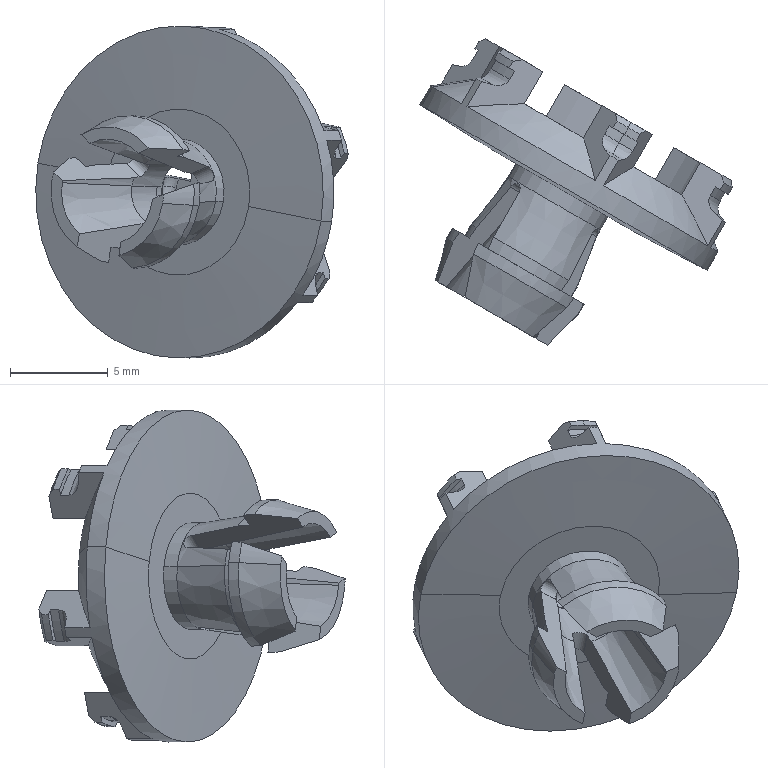Part | SolidWorks | features BaseBody 1 | 1 solid | 200 faces | box 16.002 x 15.682 x 17 mm | volume 610.766 mm3 | cylinder 63 | plane 61 | cone 52 | torus 20 | sphere 4 | commonest cylinder face diameters 0.3 x12 15 x8 15.5 x8 13 x6 6.3 x5 7.8 x5